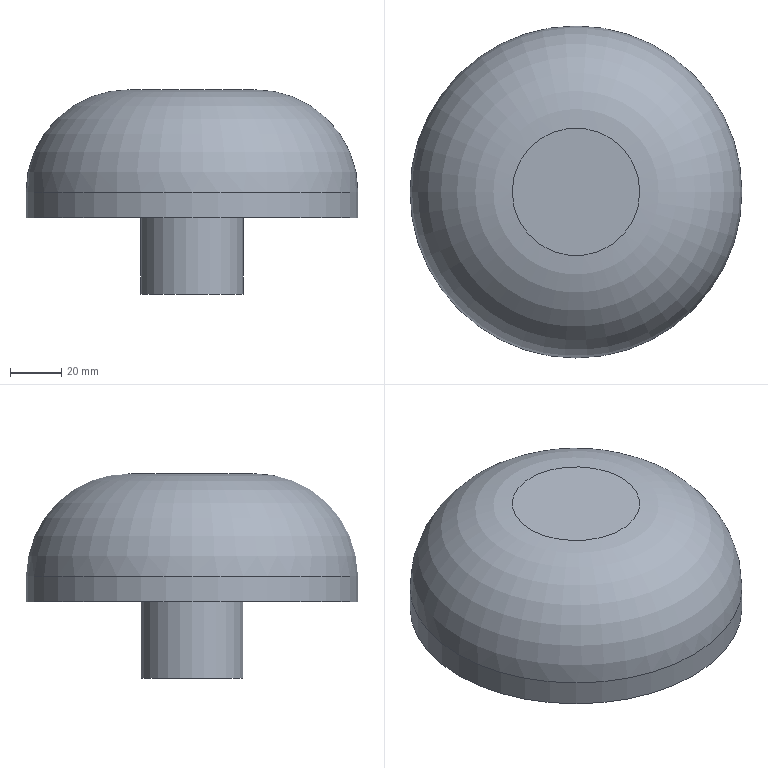Part | NX | features DATUM_CSYS 2, SKETCH 1, SWP104 1 | 1 solid | 6 faces | box 130 x 130 x 80 mm | volume 580405 mm3 | plane 3 | cylinder 2 | torus 1 | commonest cylinder face diameters 40 x1 130 x1
STEP:
#1=CARTESIAN_POINT('',(25.,0.,80.));
#2=VERTEX_POINT('',#1);
#3=CARTESIAN_POINT('',(0.,0.,80.));
#4=DIRECTION('',(0.,0.,1.));
#5=DIRECTION('',(1.,0.,0.));
#6=AXIS2_PLACEMENT_3D('',#3,#4,#5);
#7=CIRCLE('',#6,25.);
#8=EDGE_CURVE('',#2,#2,#7,.T.);
#9=ORIENTED_EDGE('',*,*,#8,.T.);
#10=EDGE_LOOP('',(#9));
#11=FACE_BOUND('',#10,.T.);
#12=CARTESIAN_POINT('',(0.,0.,80.));
#13=DIRECTION('',(0.,0.,1.));
#14=DIRECTION('',(1.,0.,0.));
#15=AXIS2_PLACEMENT_3D('',#12,#13,#14);
#16=PLANE('',#15);
#17=ADVANCED_FACE('',(#11),#16,.T.);
#18=CARTESIAN_POINT('',(65.,0.,40.));
#19=VERTEX_POINT('',#18);
#20=CARTESIAN_POINT('',(0.,0.,40.));
#21=DIRECTION('',(0.,0.,1.));
#22=DIRECTION('',(1.,0.,0.));
#23=AXIS2_PLACEMENT_3D('',#20,#21,#22);
#24=CIRCLE('',#23,65.);
#25=EDGE_CURVE('',#19,#19,#24,.T.);
#26=ORIENTED_EDGE('',*,*,#25,.T.);
#27=EDGE_LOOP('',(#26));
#28=FACE_BOUND('',#27,.T.);
#29=ORIENTED_EDGE('',*,*,#8,.F.);
#30=EDGE_LOOP('',(#29));
#31=FACE_BOUND('',#30,.T.);
#32=CARTESIAN_POINT('',(0.,0.,40.));
#33=DIRECTION('',(0.,0.,1.));
#34=DIRECTION('',(1.,0.,0.));
#35=AXIS2_PLACEMENT_3D('',#32,#33,#34);
#36=DEGENERATE_TOROIDAL_SURFACE('',#35,25.,40.,.T.);
#37=ADVANCED_FACE('',(#28,#31),#36,.T.);
#38=CARTESIAN_POINT('',(65.,0.,30.));
#39=VERTEX_POINT('',#38);
#40=CARTESIAN_POINT('',(0.,0.,30.));
#41=DIRECTION('',(0.,0.,1.));
#42=DIRECTION('',(1.,0.,0.));
#43=AXIS2_PLACEMENT_3D('',#40,#41,#42);
#44=CIRCLE('',#43,65.);
#45=EDGE_CURVE('',#39,#39,#44,.T.);
#46=ORIENTED_EDGE('',*,*,#45,.T.);
#47=EDGE_LOOP('',(#46));
#48=FACE_BOUND('',#47,.T.);
#49=ORIENTED_EDGE('',*,*,#25,.F.);
#50=EDGE_LOOP('',(#49));
#51=FACE_BOUND('',#50,.T.);
#52=CARTESIAN_POINT('',(0.,0.,0.));
#53=DIRECTION('',(0.,0.,1.));
#54=DIRECTION('',(1.,0.,0.));
#55=AXIS2_PLACEMENT_3D('',#52,#53,#54);
#56=CYLINDRICAL_SURFACE('',#55,65.);
#57=ADVANCED_FACE('',(#48,#51),#56,.T.);
#58=CARTESIAN_POINT('',(20.,0.,30.));
#59=VERTEX_POINT('',#58);
#60=CARTESIAN_POINT('',(0.,0.,30.));
#61=DIRECTION('',(0.,0.,1.));
#62=DIRECTION('',(1.,0.,0.));
#63=AXIS2_PLACEMENT_3D('',#60,#61,#62);
#64=CIRCLE('',#63,20.);
#65=EDGE_CURVE('',#59,#59,#64,.T.);
#66=ORIENTED_EDGE('',*,*,#65,.T.);
#67=EDGE_LOOP('',(#66));
#68=FACE_BOUND('',#67,.T.);
#69=ORIENTED_EDGE('',*,*,#45,.F.);
#70=EDGE_LOOP('',(#69));
#71=FACE_BOUND('',#70,.T.);
#72=CARTESIAN_POINT('',(0.,-65.,30.));
#73=DIRECTION('',(0.,0.,-1.));
#74=DIRECTION('',(-1.,0.,0.));
#75=AXIS2_PLACEMENT_3D('',#72,#73,#74);
#76=PLANE('',#75);
#77=ADVANCED_FACE('',(#68,#71),#76,.T.);
#78=CARTESIAN_POINT('',(20.,0.,0.));
#79=VERTEX_POINT('',#78);
#80=CARTESIAN_POINT('',(0.,0.,0.));
#81=DIRECTION('',(0.,0.,1.));
#82=DIRECTION('',(1.,0.,0.));
#83=AXIS2_PLACEMENT_3D('',#80,#81,#82);
#84=CIRCLE('',#83,20.);
#85=EDGE_CURVE('',#79,#79,#84,.T.);
#86=ORIENTED_EDGE('',*,*,#85,.T.);
#87=EDGE_LOOP('',(#86));
#88=FACE_BOUND('',#87,.T.);
#89=ORIENTED_EDGE('',*,*,#65,.F.);
#90=EDGE_LOOP('',(#89));
#91=FACE_BOUND('',#90,.T.);
#92=CARTESIAN_POINT('',(0.,0.,0.));
#93=DIRECTION('',(0.,0.,1.));
#94=DIRECTION('',(1.,0.,0.));
#95=AXIS2_PLACEMENT_3D('',#92,#93,#94);
#96=CYLINDRICAL_SURFACE('',#95,20.);
#97=ADVANCED_FACE('',(#88,#91),#96,.T.);
#98=ORIENTED_EDGE('',*,*,#85,.F.);
#99=EDGE_LOOP('',(#98));
#100=FACE_BOUND('',#99,.T.);
#101=CARTESIAN_POINT('',(0.,-20.,0.));
#102=DIRECTION('',(0.,0.,-1.));
#103=DIRECTION('',(-1.,0.,0.));
#104=AXIS2_PLACEMENT_3D('',#101,#102,#103);
#105=PLANE('',#104);
#106=ADVANCED_FACE('',(#100),#105,.T.);
#107=CLOSED_SHELL('',(#17,#37,#57,#77,#97,#106));
#108=MANIFOLD_SOLID_BREP('',#107);
#109=(LENGTH_UNIT()NAMED_UNIT(*)SI_UNIT(.MILLI.,.METRE.));
#110=UNCERTAINTY_MEASURE_WITH_UNIT(LENGTH_MEASURE(0.00001),#109,'','');
#111=(NAMED_UNIT(*)PLANE_ANGLE_UNIT()SI_UNIT($,.RADIAN.));
#112=(NAMED_UNIT(*)SI_UNIT($,.STERADIAN.)SOLID_ANGLE_UNIT());
#113=(GEOMETRIC_REPRESENTATION_CONTEXT(3)GLOBAL_UNCERTAINTY_ASSIGNED_CONTEXT((#110))GLOBAL_UNIT_ASSIGNED_CONTEXT((#109,#111,#112))REPRESENTATION_CONTEXT('',''));
#114=ADVANCED_BREP_SHAPE_REPRESENTATION('',(#108),#113);